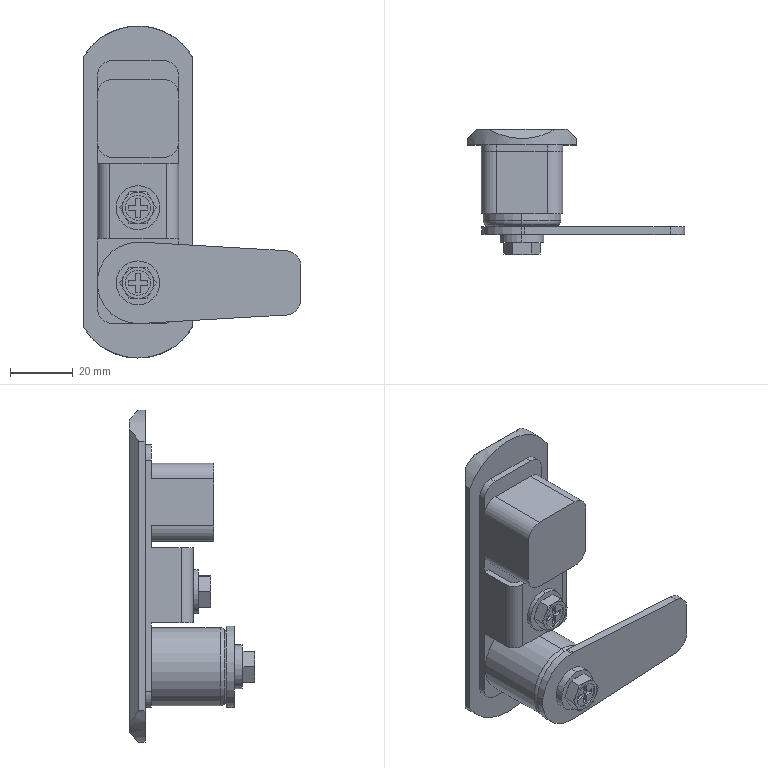Part | STEP file | 001-001-xax22-a106 | 1 solid | 162 faces | box 69.5 x 40 x 106 mm | volume 52020 mm3 | plane 90 | cylinder 44 | cone 24 | torus 4 | commonest cylinder face diameters 10 x10 4 x6 8 x6 14 x4 20.6 x3 21 x3